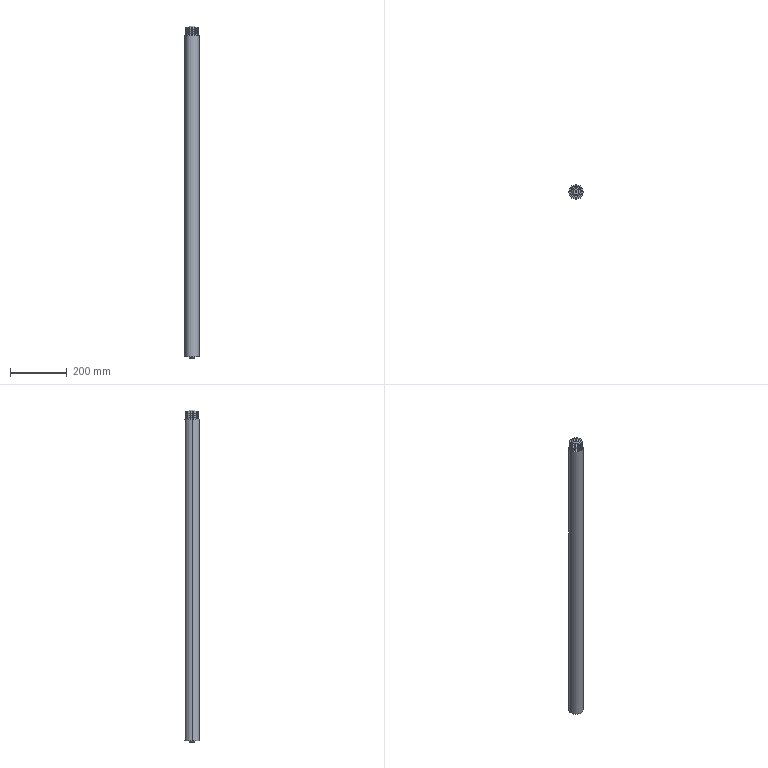Part | SolidWorks | features HoleWzd 2, ICE 2, Chamfer 1, Extrusion 1, MirrorPattern 1, RevCut 1 | 1 solid | 81 faces | box 50 x 50 x 1170 mm | volume 2265436 mm3 | cone 48 | cylinder 28 | plane 5 | commonest cylinder face diameters 43 x22 6.8 x4 50 x2